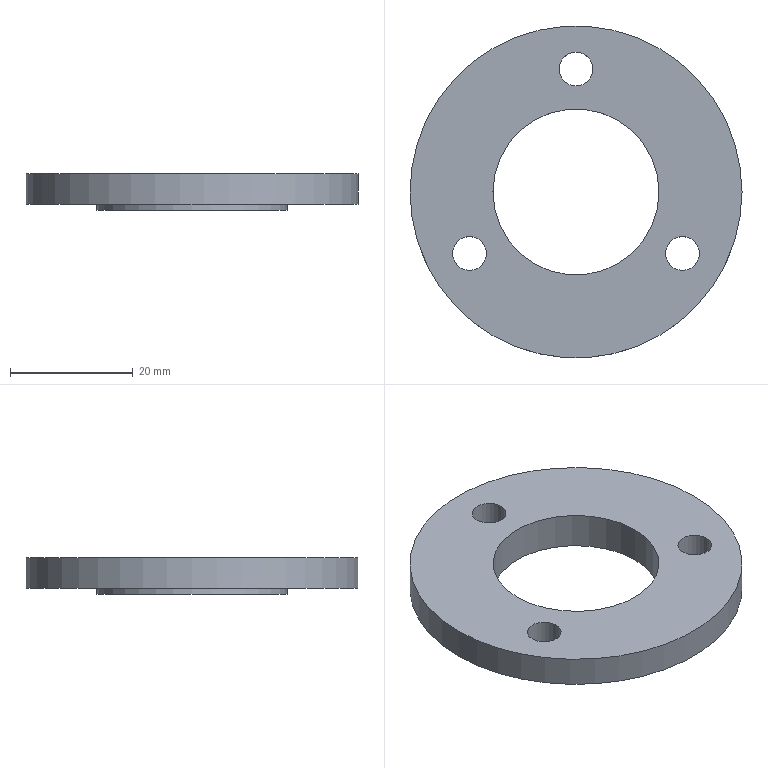Part | STEP file | YBQDJ-YL-15 | 1 solid | 9 faces | box 54 x 54 x 6 mm | volume 8414 mm3 | cylinder 6 | plane 3 | commonest cylinder face diameters 5.5 x3 27 x1 31 x1 54 x1
STEP:
#1=CARTESIAN_POINT('',(0.,0.,0.));
#2=DIRECTION('',(0.,0.,1.));
#3=DIRECTION('',(1.,0.,0.));
#4=AXIS2_PLACEMENT_3D('',#1,#2,#3);
#5=CARTESIAN_POINT('',(291.,-195.,214.));
#6=VERTEX_POINT('',#5);
#7=CARTESIAN_POINT('',(306.5,-195.,214.));
#8=DIRECTION('',(0.,0.,1.));
#9=DIRECTION('',(-1.,0.,0.));
#10=AXIS2_PLACEMENT_3D('',#7,#8,#9);
#11=CIRCLE('',#10,15.5);
#12=CARTESIAN_POINT('',(306.5,-195.,214.));
#13=DIRECTION('',(0.,0.,1.));
#14=DIRECTION('',(-1.,0.,0.));
#15=AXIS2_PLACEMENT_3D('',#12,#13,#14);
#16=PLANE('',#15);
#17=CARTESIAN_POINT('',(0.,0.));
#18=DIRECTION('',(1.,0.));
#19=AXIS2_PLACEMENT_2D('',#17,#18);
#20=CIRCLE('',#19,15.5);
#21=(GEOMETRIC_REPRESENTATION_CONTEXT(2)PARAMETRIC_REPRESENTATION_CONTEXT()REPRESENTATION_CONTEXT('',''));
#22=DEFINITIONAL_REPRESENTATION('',(#20),#21);
#23=PCURVE('',#16,#22);
#24=CARTESIAN_POINT('',(306.5,-195.,214.));
#25=DIRECTION('',(0.,0.,-1.));
#26=DIRECTION('',(-1.,0.,0.));
#27=AXIS2_PLACEMENT_3D('',#24,#25,#26);
#28=CYLINDRICAL_SURFACE('',#27,15.5);
#29=CARTESIAN_POINT('',(6.283,0.));
#30=DIRECTION('',(-1.,0.));
#31=VECTOR('',#30,1.);
#32=LINE('',#29,#31);
#33=(GEOMETRIC_REPRESENTATION_CONTEXT(2)PARAMETRIC_REPRESENTATION_CONTEXT()REPRESENTATION_CONTEXT('',''));
#34=DEFINITIONAL_REPRESENTATION('',(#32),#33);
#35=PCURVE('',#28,#34);
#36=SURFACE_CURVE('',#11,(#23,#35),.PCURVE_S1.);
#37=EDGE_CURVE('',#6,#6,#36,.T.);
#38=ORIENTED_EDGE('',*,*,#37,.T.);
#39=EDGE_LOOP('',(#38));
#40=FACE_BOUND('',#39,.T.);
#41=CARTESIAN_POINT('',(303.75,-175.,214.));
#42=VERTEX_POINT('',#41);
#43=CARTESIAN_POINT('',(306.5,-175.,214.));
#44=DIRECTION('',(0.,0.,1.));
#45=DIRECTION('',(-1.,0.,0.));
#46=AXIS2_PLACEMENT_3D('',#43,#44,#45);
#47=CIRCLE('',#46,2.75);
#48=CARTESIAN_POINT('',(0.,-20.));
#49=DIRECTION('',(1.,0.));
#50=AXIS2_PLACEMENT_2D('',#48,#49);
#51=CIRCLE('',#50,2.75);
#52=(GEOMETRIC_REPRESENTATION_CONTEXT(2)PARAMETRIC_REPRESENTATION_CONTEXT()REPRESENTATION_CONTEXT('',''));
#53=DEFINITIONAL_REPRESENTATION('',(#51),#52);
#54=PCURVE('',#16,#53);
#55=CARTESIAN_POINT('',(306.5,-175.,224.));
#56=DIRECTION('',(0.,0.,-1.));
#57=DIRECTION('',(1.,0.,0.));
#58=AXIS2_PLACEMENT_3D('',#55,#56,#57);
#59=CYLINDRICAL_SURFACE('',#58,2.75);
#60=CARTESIAN_POINT('',(9.425,10.));
#61=DIRECTION('',(-1.,0.));
#62=VECTOR('',#61,1.);
#63=LINE('',#60,#62);
#64=(GEOMETRIC_REPRESENTATION_CONTEXT(2)PARAMETRIC_REPRESENTATION_CONTEXT()REPRESENTATION_CONTEXT('',''));
#65=DEFINITIONAL_REPRESENTATION('',(#63),#64);
#66=PCURVE('',#59,#65);
#67=SURFACE_CURVE('',#47,(#54,#66),.PCURVE_S1.);
#68=EDGE_CURVE('',#42,#42,#67,.T.);
#69=ORIENTED_EDGE('',*,*,#68,.T.);
#70=EDGE_LOOP('',(#69));
#71=FACE_BOUND('',#70,.T.);
#72=CARTESIAN_POINT('',(286.429,-205.,214.));
#73=VERTEX_POINT('',#72);
#74=CARTESIAN_POINT('',(289.179,-205.,214.));
#75=DIRECTION('',(0.,0.,1.));
#76=DIRECTION('',(-1.,0.,0.));
#77=AXIS2_PLACEMENT_3D('',#74,#75,#76);
#78=CIRCLE('',#77,2.75);
#79=CARTESIAN_POINT('',(17.321,10.));
#80=DIRECTION('',(1.,0.));
#81=AXIS2_PLACEMENT_2D('',#79,#80);
#82=CIRCLE('',#81,2.75);
#83=(GEOMETRIC_REPRESENTATION_CONTEXT(2)PARAMETRIC_REPRESENTATION_CONTEXT()REPRESENTATION_CONTEXT('',''));
#84=DEFINITIONAL_REPRESENTATION('',(#82),#83);
#85=PCURVE('',#16,#84);
#86=CARTESIAN_POINT('',(289.179,-205.,224.));
#87=DIRECTION('',(0.,0.,-1.));
#88=DIRECTION('',(1.,0.,0.));
#89=AXIS2_PLACEMENT_3D('',#86,#87,#88);
#90=CYLINDRICAL_SURFACE('',#89,2.75);
#91=CARTESIAN_POINT('',(9.425,10.));
#92=DIRECTION('',(-1.,0.));
#93=VECTOR('',#92,1.);
#94=LINE('',#91,#93);
#95=(GEOMETRIC_REPRESENTATION_CONTEXT(2)PARAMETRIC_REPRESENTATION_CONTEXT()REPRESENTATION_CONTEXT('',''));
#96=DEFINITIONAL_REPRESENTATION('',(#94),#95);
#97=PCURVE('',#90,#96);
#98=SURFACE_CURVE('',#78,(#85,#97),.PCURVE_S1.);
#99=EDGE_CURVE('',#73,#73,#98,.T.);
#100=ORIENTED_EDGE('',*,*,#99,.T.);
#101=EDGE_LOOP('',(#100));
#102=FACE_BOUND('',#101,.T.);
#103=CARTESIAN_POINT('',(321.071,-205.,214.));
#104=VERTEX_POINT('',#103);
#105=CARTESIAN_POINT('',(323.821,-205.,214.));
#106=DIRECTION('',(0.,0.,1.));
#107=DIRECTION('',(-1.,0.,0.));
#108=AXIS2_PLACEMENT_3D('',#105,#106,#107);
#109=CIRCLE('',#108,2.75);
#110=CARTESIAN_POINT('',(-17.321,10.));
#111=DIRECTION('',(1.,0.));
#112=AXIS2_PLACEMENT_2D('',#110,#111);
#113=CIRCLE('',#112,2.75);
#114=(GEOMETRIC_REPRESENTATION_CONTEXT(2)PARAMETRIC_REPRESENTATION_CONTEXT()REPRESENTATION_CONTEXT('',''));
#115=DEFINITIONAL_REPRESENTATION('',(#113),#114);
#116=PCURVE('',#16,#115);
#117=CARTESIAN_POINT('',(323.821,-205.,224.));
#118=DIRECTION('',(0.,0.,-1.));
#119=DIRECTION('',(1.,0.,0.));
#120=AXIS2_PLACEMENT_3D('',#117,#118,#119);
#121=CYLINDRICAL_SURFACE('',#120,2.75);
#122=CARTESIAN_POINT('',(9.425,10.));
#123=DIRECTION('',(-1.,0.));
#124=VECTOR('',#123,1.);
#125=LINE('',#122,#124);
#126=(GEOMETRIC_REPRESENTATION_CONTEXT(2)PARAMETRIC_REPRESENTATION_CONTEXT()REPRESENTATION_CONTEXT('',''));
#127=DEFINITIONAL_REPRESENTATION('',(#125),#126);
#128=PCURVE('',#121,#127);
#129=SURFACE_CURVE('',#109,(#116,#128),.PCURVE_S1.);
#130=EDGE_CURVE('',#104,#104,#129,.T.);
#131=ORIENTED_EDGE('',*,*,#130,.T.);
#132=EDGE_LOOP('',(#131));
#133=FACE_BOUND('',#132,.T.);
#134=CARTESIAN_POINT('',(333.5,-195.,214.));
#135=VERTEX_POINT('',#134);
#136=CARTESIAN_POINT('',(306.5,-195.,214.));
#137=DIRECTION('',(0.,0.,-1.));
#138=DIRECTION('',(1.,0.,0.));
#139=AXIS2_PLACEMENT_3D('',#136,#137,#138);
#140=CIRCLE('',#139,27.);
#141=CARTESIAN_POINT('',(-27.,0.));
#142=CARTESIAN_POINT('',(-27.,46.765));
#143=CARTESIAN_POINT('',(13.5,23.383));
#144=CARTESIAN_POINT('',(54.,0.));
#145=CARTESIAN_POINT('',(13.5,-23.383));
#146=CARTESIAN_POINT('',(-27.,-46.765));
#147=CARTESIAN_POINT('',(-27.,0.));
#148=(BOUNDED_CURVE()B_SPLINE_CURVE(2,(#141,#142,#143,#144,#145,#146,#147),.UNSPECIFIED.,.T.,.F.)B_SPLINE_CURVE_WITH_KNOTS((1,2,2,2,2,1),(-2.094,0.,2.094,4.189,6.283,8.378),.UNSPECIFIED.)CURVE()GEOMETRIC_REPRESENTATION_ITEM()RATIONAL_B_SPLINE_CURVE((1.,0.5,1.,0.5,1.,0.5,1.))REPRESENTATION_ITEM(''));
#149=(GEOMETRIC_REPRESENTATION_CONTEXT(2)PARAMETRIC_REPRESENTATION_CONTEXT()REPRESENTATION_CONTEXT('',''));
#150=DEFINITIONAL_REPRESENTATION('',(#148),#149);
#151=PCURVE('',#16,#150);
#152=CARTESIAN_POINT('',(306.5,-195.,214.));
#153=DIRECTION('',(0.,0.,1.));
#154=DIRECTION('',(-1.,0.,0.));
#155=AXIS2_PLACEMENT_3D('',#152,#153,#154);
#156=CYLINDRICAL_SURFACE('',#155,27.);
#157=CARTESIAN_POINT('',(9.425,0.));
#158=DIRECTION('',(-1.,0.));
#159=VECTOR('',#158,1.);
#160=LINE('',#157,#159);
#161=(GEOMETRIC_REPRESENTATION_CONTEXT(2)PARAMETRIC_REPRESENTATION_CONTEXT()REPRESENTATION_CONTEXT('',''));
#162=DEFINITIONAL_REPRESENTATION('',(#160),#161);
#163=PCURVE('',#156,#162);
#164=SURFACE_CURVE('',#140,(#151,#163),.PCURVE_S1.);
#165=EDGE_CURVE('',#135,#135,#164,.T.);
#166=ORIENTED_EDGE('',*,*,#165,.T.);
#167=EDGE_LOOP('',(#166));
#168=FACE_BOUND('',#167,.T.);
#169=ADVANCED_FACE('',(#40,#71,#102,#133,#168),#16,.F.);
#170=CARTESIAN_POINT('',(303.75,-175.,219.));
#171=VERTEX_POINT('',#170);
#172=CARTESIAN_POINT('',(306.5,-175.,219.));
#173=DIRECTION('',(0.,0.,-1.));
#174=DIRECTION('',(-1.,0.,0.));
#175=AXIS2_PLACEMENT_3D('',#172,#173,#174);
#176=CIRCLE('',#175,2.75);
#177=CARTESIAN_POINT('',(306.5,-195.,219.));
#178=DIRECTION('',(0.,0.,1.));
#179=DIRECTION('',(-1.,0.,0.));
#180=AXIS2_PLACEMENT_3D('',#177,#178,#179);
#181=PLANE('',#180);
#182=CARTESIAN_POINT('',(2.75,-20.));
#183=CARTESIAN_POINT('',(2.75,-24.763));
#184=CARTESIAN_POINT('',(-1.375,-22.382));
#185=CARTESIAN_POINT('',(-5.5,-20.));
#186=CARTESIAN_POINT('',(-1.375,-17.618));
#187=CARTESIAN_POINT('',(2.75,-15.237));
#188=CARTESIAN_POINT('',(2.75,-20.));
#189=(BOUNDED_CURVE()B_SPLINE_CURVE(2,(#182,#183,#184,#185,#186,#187,#188),.UNSPECIFIED.,.T.,.F.)B_SPLINE_CURVE_WITH_KNOTS((1,2,2,2,2,1),(-2.094,0.,2.094,4.189,6.283,8.378),.UNSPECIFIED.)CURVE()GEOMETRIC_REPRESENTATION_ITEM()RATIONAL_B_SPLINE_CURVE((1.,0.5,1.,0.5,1.,0.5,1.))REPRESENTATION_ITEM(''));
#190=(GEOMETRIC_REPRESENTATION_CONTEXT(2)PARAMETRIC_REPRESENTATION_CONTEXT()REPRESENTATION_CONTEXT('',''));
#191=DEFINITIONAL_REPRESENTATION('',(#189),#190);
#192=PCURVE('',#181,#191);
#193=CARTESIAN_POINT('',(3.142,5.));
#194=DIRECTION('',(1.,0.));
#195=VECTOR('',#194,1.);
#196=LINE('',#193,#195);
#197=(GEOMETRIC_REPRESENTATION_CONTEXT(2)PARAMETRIC_REPRESENTATION_CONTEXT()REPRESENTATION_CONTEXT('',''));
#198=DEFINITIONAL_REPRESENTATION('',(#196),#197);
#199=PCURVE('',#59,#198);
#200=SURFACE_CURVE('',#176,(#192,#199),.PCURVE_S1.);
#201=EDGE_CURVE('',#171,#171,#200,.T.);
#202=ORIENTED_EDGE('',*,*,#201,.T.);
#203=EDGE_LOOP('',(#202));
#204=FACE_BOUND('',#203,.T.);
#205=CARTESIAN_POINT('',(286.429,-205.,219.));
#206=VERTEX_POINT('',#205);
#207=CARTESIAN_POINT('',(289.179,-205.,219.));
#208=DIRECTION('',(0.,0.,-1.));
#209=DIRECTION('',(-1.,0.,0.));
#210=AXIS2_PLACEMENT_3D('',#207,#208,#209);
#211=CIRCLE('',#210,2.75);
#212=CARTESIAN_POINT('',(20.071,10.));
#213=CARTESIAN_POINT('',(20.071,5.237));
#214=CARTESIAN_POINT('',(15.946,7.618));
#215=CARTESIAN_POINT('',(11.821,10.));
#216=CARTESIAN_POINT('',(15.946,12.382));
#217=CARTESIAN_POINT('',(20.071,14.763));
#218=CARTESIAN_POINT('',(20.071,10.));
#219=(BOUNDED_CURVE()B_SPLINE_CURVE(2,(#212,#213,#214,#215,#216,#217,#218),.UNSPECIFIED.,.T.,.F.)B_SPLINE_CURVE_WITH_KNOTS((1,2,2,2,2,1),(-2.094,0.,2.094,4.189,6.283,8.378),.UNSPECIFIED.)CURVE()GEOMETRIC_REPRESENTATION_ITEM()RATIONAL_B_SPLINE_CURVE((1.,0.5,1.,0.5,1.,0.5,1.))REPRESENTATION_ITEM(''));
#220=(GEOMETRIC_REPRESENTATION_CONTEXT(2)PARAMETRIC_REPRESENTATION_CONTEXT()REPRESENTATION_CONTEXT('',''));
#221=DEFINITIONAL_REPRESENTATION('',(#219),#220);
#222=PCURVE('',#181,#221);
#223=CARTESIAN_POINT('',(3.142,5.));
#224=DIRECTION('',(1.,0.));
#225=VECTOR('',#224,1.);
#226=LINE('',#223,#225);
#227=(GEOMETRIC_REPRESENTATION_CONTEXT(2)PARAMETRIC_REPRESENTATION_CONTEXT()REPRESENTATION_CONTEXT('',''));
#228=DEFINITIONAL_REPRESENTATION('',(#226),#227);
#229=PCURVE('',#90,#228);
#230=SURFACE_CURVE('',#211,(#222,#229),.PCURVE_S1.);
#231=EDGE_CURVE('',#206,#206,#230,.T.);
#232=ORIENTED_EDGE('',*,*,#231,.T.);
#233=EDGE_LOOP('',(#232));
#234=FACE_BOUND('',#233,.T.);
#235=CARTESIAN_POINT('',(321.071,-205.,219.));
#236=VERTEX_POINT('',#235);
#237=CARTESIAN_POINT('',(323.821,-205.,219.));
#238=DIRECTION('',(0.,0.,-1.));
#239=DIRECTION('',(-1.,0.,0.));
#240=AXIS2_PLACEMENT_3D('',#237,#238,#239);
#241=CIRCLE('',#240,2.75);
#242=CARTESIAN_POINT('',(-14.571,10.));
#243=CARTESIAN_POINT('',(-14.571,5.237));
#244=CARTESIAN_POINT('',(-18.696,7.618));
#245=CARTESIAN_POINT('',(-22.821,10.));
#246=CARTESIAN_POINT('',(-18.696,12.382));
#247=CARTESIAN_POINT('',(-14.571,14.763));
#248=CARTESIAN_POINT('',(-14.571,10.));
#249=(BOUNDED_CURVE()B_SPLINE_CURVE(2,(#242,#243,#244,#245,#246,#247,#248),.UNSPECIFIED.,.T.,.F.)B_SPLINE_CURVE_WITH_KNOTS((1,2,2,2,2,1),(-2.094,0.,2.094,4.189,6.283,8.378),.UNSPECIFIED.)CURVE()GEOMETRIC_REPRESENTATION_ITEM()RATIONAL_B_SPLINE_CURVE((1.,0.5,1.,0.5,1.,0.5,1.))REPRESENTATION_ITEM(''));
#250=(GEOMETRIC_REPRESENTATION_CONTEXT(2)PARAMETRIC_REPRESENTATION_CONTEXT()REPRESENTATION_CONTEXT('',''));
#251=DEFINITIONAL_REPRESENTATION('',(#249),#250);
#252=PCURVE('',#181,#251);
#253=CARTESIAN_POINT('',(3.142,5.));
#254=DIRECTION('',(1.,0.));
#255=VECTOR('',#254,1.);
#256=LINE('',#253,#255);
#257=(GEOMETRIC_REPRESENTATION_CONTEXT(2)PARAMETRIC_REPRESENTATION_CONTEXT()REPRESENTATION_CONTEXT('',''));
#258=DEFINITIONAL_REPRESENTATION('',(#256),#257);
#259=PCURVE('',#121,#258);
#260=SURFACE_CURVE('',#241,(#252,#259),.PCURVE_S1.);
#261=EDGE_CURVE('',#236,#236,#260,.T.);
#262=ORIENTED_EDGE('',*,*,#261,.T.);
#263=EDGE_LOOP('',(#262));
#264=FACE_BOUND('',#263,.T.);
#265=CARTESIAN_POINT('',(333.5,-195.,219.));
#266=VERTEX_POINT('',#265);
#267=CARTESIAN_POINT('',(306.5,-195.,219.));
#268=DIRECTION('',(0.,0.,-1.));
#269=DIRECTION('',(1.,0.,0.));
#270=AXIS2_PLACEMENT_3D('',#267,#268,#269);
#271=CIRCLE('',#270,27.);
#272=CARTESIAN_POINT('',(-27.,0.));
#273=CARTESIAN_POINT('',(-27.,46.765));
#274=CARTESIAN_POINT('',(13.5,23.383));
#275=CARTESIAN_POINT('',(54.,0.));
#276=CARTESIAN_POINT('',(13.5,-23.383));
#277=CARTESIAN_POINT('',(-27.,-46.765));
#278=CARTESIAN_POINT('',(-27.,0.));
#279=(BOUNDED_CURVE()B_SPLINE_CURVE(2,(#272,#273,#274,#275,#276,#277,#278),.UNSPECIFIED.,.T.,.F.)B_SPLINE_CURVE_WITH_KNOTS((1,2,2,2,2,1),(-2.094,0.,2.094,4.189,6.283,8.378),.UNSPECIFIED.)CURVE()GEOMETRIC_REPRESENTATION_ITEM()RATIONAL_B_SPLINE_CURVE((1.,0.5,1.,0.5,1.,0.5,1.))REPRESENTATION_ITEM(''));
#280=(GEOMETRIC_REPRESENTATION_CONTEXT(2)PARAMETRIC_REPRESENTATION_CONTEXT()REPRESENTATION_CONTEXT('',''));
#281=DEFINITIONAL_REPRESENTATION('',(#279),#280);
#282=PCURVE('',#181,#281);
#283=CARTESIAN_POINT('',(9.425,5.));
#284=DIRECTION('',(-1.,0.));
#285=VECTOR('',#284,1.);
#286=LINE('',#283,#285);
#287=(GEOMETRIC_REPRESENTATION_CONTEXT(2)PARAMETRIC_REPRESENTATION_CONTEXT()REPRESENTATION_CONTEXT('',''));
#288=DEFINITIONAL_REPRESENTATION('',(#286),#287);
#289=PCURVE('',#156,#288);
#290=SURFACE_CURVE('',#271,(#282,#289),.PCURVE_S1.);
#291=EDGE_CURVE('',#266,#266,#290,.T.);
#292=ORIENTED_EDGE('',*,*,#291,.F.);
#293=EDGE_LOOP('',(#292));
#294=FACE_BOUND('',#293,.T.);
#295=CARTESIAN_POINT('',(320.,-195.,219.));
#296=VERTEX_POINT('',#295);
#297=CARTESIAN_POINT('',(293.,-195.,219.));
#298=VERTEX_POINT('',#297);
#299=CARTESIAN_POINT('',(306.5,-195.,219.));
#300=DIRECTION('',(0.,0.,-1.));
#301=DIRECTION('',(1.,0.,0.));
#302=AXIS2_PLACEMENT_3D('',#299,#300,#301);
#303=CIRCLE('',#302,13.5);
#304=CARTESIAN_POINT('',(-13.5,0.));
#305=CARTESIAN_POINT('',(-13.5,23.383));
#306=CARTESIAN_POINT('',(6.75,11.691));
#307=CARTESIAN_POINT('',(27.,0.));
#308=CARTESIAN_POINT('',(6.75,-11.691));
#309=CARTESIAN_POINT('',(-13.5,-23.383));
#310=CARTESIAN_POINT('',(-13.5,0.));
#311=(BOUNDED_CURVE()B_SPLINE_CURVE(2,(#304,#305,#306,#307,#308,#309,#310),.UNSPECIFIED.,.T.,.F.)B_SPLINE_CURVE_WITH_KNOTS((1,2,2,2,2,1),(-2.094,0.,2.094,4.189,6.283,8.378),.UNSPECIFIED.)CURVE()GEOMETRIC_REPRESENTATION_ITEM()RATIONAL_B_SPLINE_CURVE((1.,0.5,1.,0.5,1.,0.5,1.))REPRESENTATION_ITEM(''));
#312=(GEOMETRIC_REPRESENTATION_CONTEXT(2)PARAMETRIC_REPRESENTATION_CONTEXT()REPRESENTATION_CONTEXT('',''));
#313=DEFINITIONAL_REPRESENTATION('',(#311),#312);
#314=PCURVE('',#181,#313);
#315=CARTESIAN_POINT('',(306.5,-195.,214.));
#316=DIRECTION('',(0.,0.,1.));
#317=DIRECTION('',(-1.,0.,0.));
#318=AXIS2_PLACEMENT_3D('',#315,#316,#317);
#319=CYLINDRICAL_SURFACE('',#318,13.5);
#320=CARTESIAN_POINT('',(3.142,5.));
#321=DIRECTION('',(-1.,0.));
#322=VECTOR('',#321,1.);
#323=LINE('',#320,#322);
#324=(GEOMETRIC_REPRESENTATION_CONTEXT(2)PARAMETRIC_REPRESENTATION_CONTEXT()REPRESENTATION_CONTEXT('',''));
#325=DEFINITIONAL_REPRESENTATION('',(#323),#324);
#326=PCURVE('',#319,#325);
#327=SURFACE_CURVE('',#303,(#314,#326),.PCURVE_S1.);
#328=EDGE_CURVE('',#296,#298,#327,.T.);
#329=ORIENTED_EDGE('',*,*,#328,.T.);
#330=CARTESIAN_POINT('',(306.5,-195.,219.));
#331=DIRECTION('',(0.,0.,-1.));
#332=DIRECTION('',(1.,0.,0.));
#333=AXIS2_PLACEMENT_3D('',#330,#331,#332);
#334=CIRCLE('',#333,13.5);
#335=CARTESIAN_POINT('',(-13.5,0.));
#336=CARTESIAN_POINT('',(-13.5,23.383));
#337=CARTESIAN_POINT('',(6.75,11.691));
#338=CARTESIAN_POINT('',(27.,0.));
#339=CARTESIAN_POINT('',(6.75,-11.691));
#340=CARTESIAN_POINT('',(-13.5,-23.383));
#341=CARTESIAN_POINT('',(-13.5,0.));
#342=(BOUNDED_CURVE()B_SPLINE_CURVE(2,(#335,#336,#337,#338,#339,#340,#341),.UNSPECIFIED.,.T.,.F.)B_SPLINE_CURVE_WITH_KNOTS((1,2,2,2,2,1),(-2.094,0.,2.094,4.189,6.283,8.378),.UNSPECIFIED.)CURVE()GEOMETRIC_REPRESENTATION_ITEM()RATIONAL_B_SPLINE_CURVE((1.,0.5,1.,0.5,1.,0.5,1.))REPRESENTATION_ITEM(''));
#343=(GEOMETRIC_REPRESENTATION_CONTEXT(2)PARAMETRIC_REPRESENTATION_CONTEXT()REPRESENTATION_CONTEXT('',''));
#344=DEFINITIONAL_REPRESENTATION('',(#342),#343);
#345=PCURVE('',#181,#344);
#346=CARTESIAN_POINT('',(9.425,5.));
#347=DIRECTION('',(-1.,0.));
#348=VECTOR('',#347,1.);
#349=LINE('',#346,#348);
#350=(GEOMETRIC_REPRESENTATION_CONTEXT(2)PARAMETRIC_REPRESENTATION_CONTEXT()REPRESENTATION_CONTEXT('',''));
#351=DEFINITIONAL_REPRESENTATION('',(#349),#350);
#352=PCURVE('',#319,#351);
#353=SURFACE_CURVE('',#334,(#345,#352),.PCURVE_S1.);
#354=EDGE_CURVE('',#298,#296,#353,.T.);
#355=ORIENTED_EDGE('',*,*,#354,.T.);
#356=EDGE_LOOP('',(#329,#355));
#357=FACE_BOUND('',#356,.T.);
#358=ADVANCED_FACE('',(#204,#234,#264,#294,#357),#181,.T.);
#359=ORIENTED_EDGE('',*,*,#165,.F.);
#360=CARTESIAN_POINT('',(333.5,-195.,214.));
#361=CARTESIAN_POINT('',(333.5,-195.,219.));
#362=B_SPLINE_CURVE_WITH_KNOTS('',1,(#360,#361),.UNSPECIFIED.,.F.,.F.,(2,2),(0.,5.),.PIECEWISE_BEZIER_KNOTS.);
#363=CARTESIAN_POINT('',(9.425,0.));
#364=DIRECTION('',(0.,1.));
#365=VECTOR('',#364,1.);
#366=LINE('',#363,#365);
#367=(GEOMETRIC_REPRESENTATION_CONTEXT(2)PARAMETRIC_REPRESENTATION_CONTEXT()REPRESENTATION_CONTEXT('',''));
#368=DEFINITIONAL_REPRESENTATION('',(#366),#367);
#369=PCURVE('',#156,#368);
#370=CARTESIAN_POINT('',(3.142,0.));
#371=DIRECTION('',(0.,1.));
#372=VECTOR('',#371,1.);
#373=LINE('',#370,#372);
#374=(GEOMETRIC_REPRESENTATION_CONTEXT(2)PARAMETRIC_REPRESENTATION_CONTEXT()REPRESENTATION_CONTEXT('',''));
#375=DEFINITIONAL_REPRESENTATION('',(#373),#374);
#376=PCURVE('',#156,#375);
#377=SEAM_CURVE('',#362,(#369,#376),.PCURVE_S1.);
#378=EDGE_CURVE('',#135,#266,#377,.T.);
#379=ORIENTED_EDGE('',*,*,#378,.T.);
#380=ORIENTED_EDGE('',*,*,#291,.T.);
#381=ORIENTED_EDGE('',*,*,#378,.F.);
#382=EDGE_LOOP('',(#359,#379,#380,#381));
#383=FACE_BOUND('',#382,.T.);
#384=ADVANCED_FACE('',(#383),#156,.T.);
#385=ORIENTED_EDGE('',*,*,#328,.T.);
#386=CARTESIAN_POINT('',(293.,-195.,213.));
#387=VERTEX_POINT('',#386);
#388=CARTESIAN_POINT('',(293.,-195.,213.));
#389=CARTESIAN_POINT('',(293.,-195.,219.));
#390=B_SPLINE_CURVE_WITH_KNOTS('',1,(#388,#389),.UNSPECIFIED.,.F.,.F.,(2,2),(-1.,5.),.PIECEWISE_BEZIER_KNOTS.);
#391=CARTESIAN_POINT('',(0.,0.));
#392=DIRECTION('',(0.,1.));
#393=VECTOR('',#392,1.);
#394=LINE('',#391,#393);
#395=(GEOMETRIC_REPRESENTATION_CONTEXT(2)PARAMETRIC_REPRESENTATION_CONTEXT()REPRESENTATION_CONTEXT('',''));
#396=DEFINITIONAL_REPRESENTATION('',(#394),#395);
#397=PCURVE('',#319,#396);
#398=CARTESIAN_POINT('',(6.283,0.));
#399=DIRECTION('',(0.,1.));
#400=VECTOR('',#399,1.);
#401=LINE('',#398,#400);
#402=(GEOMETRIC_REPRESENTATION_CONTEXT(2)PARAMETRIC_REPRESENTATION_CONTEXT()REPRESENTATION_CONTEXT('',''));
#403=DEFINITIONAL_REPRESENTATION('',(#401),#402);
#404=PCURVE('',#319,#403);
#405=SEAM_CURVE('',#390,(#397,#404),.PCURVE_S1.);
#406=EDGE_CURVE('',#387,#298,#405,.T.);
#407=ORIENTED_EDGE('',*,*,#406,.F.);
#408=CARTESIAN_POINT('',(306.5,-195.,213.));
#409=DIRECTION('',(0.,0.,1.));
#410=DIRECTION('',(-1.,0.,0.));
#411=AXIS2_PLACEMENT_3D('',#408,#409,#410);
#412=CIRCLE('',#411,13.5);
#413=CARTESIAN_POINT('',(0.,-1.));
#414=DIRECTION('',(1.,0.));
#415=VECTOR('',#414,1.);
#416=LINE('',#413,#415);
#417=(GEOMETRIC_REPRESENTATION_CONTEXT(2)PARAMETRIC_REPRESENTATION_CONTEXT()REPRESENTATION_CONTEXT('',''));
#418=DEFINITIONAL_REPRESENTATION('',(#416),#417);
#419=PCURVE('',#319,#418);
#420=CARTESIAN_POINT('',(306.5,-195.,213.));
#421=DIRECTION('',(0.,0.,-1.));
#422=DIRECTION('',(-1.,0.,0.));
#423=AXIS2_PLACEMENT_3D('',#420,#421,#422);
#424=PLANE('',#423);
#425=CARTESIAN_POINT('',(13.5,0.));
#426=CARTESIAN_POINT('',(13.5,-23.383));
#427=CARTESIAN_POINT('',(-6.75,-11.691));
#428=CARTESIAN_POINT('',(-27.,0.));
#429=CARTESIAN_POINT('',(-6.75,11.691));
#430=CARTESIAN_POINT('',(13.5,23.383));
#431=CARTESIAN_POINT('',(13.5,0.));
#432=(BOUNDED_CURVE()B_SPLINE_CURVE(2,(#425,#426,#427,#428,#429,#430,#431),.UNSPECIFIED.,.T.,.F.)B_SPLINE_CURVE_WITH_KNOTS((1,2,2,2,2,1),(-2.094,0.,2.094,4.189,6.283,8.378),.UNSPECIFIED.)CURVE()GEOMETRIC_REPRESENTATION_ITEM()RATIONAL_B_SPLINE_CURVE((1.,0.5,1.,0.5,1.,0.5,1.))REPRESENTATION_ITEM(''));
#433=(GEOMETRIC_REPRESENTATION_CONTEXT(2)PARAMETRIC_REPRESENTATION_CONTEXT()REPRESENTATION_CONTEXT('',''));
#434=DEFINITIONAL_REPRESENTATION('',(#432),#433);
#435=PCURVE('',#424,#434);
#436=SURFACE_CURVE('',#412,(#419,#435),.PCURVE_S1.);
#437=EDGE_CURVE('',#387,#387,#436,.T.);
#438=ORIENTED_EDGE('',*,*,#437,.T.);
#439=ORIENTED_EDGE('',*,*,#406,.T.);
#440=ORIENTED_EDGE('',*,*,#354,.T.);
#441=EDGE_LOOP('',(#385,#407,#438,#439,#440));
#442=FACE_BOUND('',#441,.F.);
#443=ADVANCED_FACE('',(#442),#319,.F.);
#444=ORIENTED_EDGE('',*,*,#130,.T.);
#445=CARTESIAN_POINT('',(321.071,-205.,219.));
#446=CARTESIAN_POINT('',(321.071,-205.,214.));
#447=B_SPLINE_CURVE_WITH_KNOTS('',1,(#445,#446),.UNSPECIFIED.,.F.,.F.,(2,2),(5.,10.),.PIECEWISE_BEZIER_KNOTS.);
#448=CARTESIAN_POINT('',(3.142,0.));
#449=DIRECTION('',(0.,1.));
#450=VECTOR('',#449,1.);
#451=LINE('',#448,#450);
#452=(GEOMETRIC_REPRESENTATION_CONTEXT(2)PARAMETRIC_REPRESENTATION_CONTEXT()REPRESENTATION_CONTEXT('',''));
#453=DEFINITIONAL_REPRESENTATION('',(#451),#452);
#454=PCURVE('',#121,#453);
#455=CARTESIAN_POINT('',(9.425,0.));
#456=DIRECTION('',(0.,1.));
#457=VECTOR('',#456,1.);
#458=LINE('',#455,#457);
#459=(GEOMETRIC_REPRESENTATION_CONTEXT(2)PARAMETRIC_REPRESENTATION_CONTEXT()REPRESENTATION_CONTEXT('',''));
#460=DEFINITIONAL_REPRESENTATION('',(#458),#459);
#461=PCURVE('',#121,#460);
#462=SEAM_CURVE('',#447,(#454,#461),.PCURVE_S1.);
#463=EDGE_CURVE('',#236,#104,#462,.T.);
#464=ORIENTED_EDGE('',*,*,#463,.F.);
#465=ORIENTED_EDGE('',*,*,#261,.T.);
#466=ORIENTED_EDGE('',*,*,#463,.T.);
#467=EDGE_LOOP('',(#444,#464,#465,#466));
#468=FACE_BOUND('',#467,.F.);
#469=ADVANCED_FACE('',(#468),#121,.F.);
#470=ORIENTED_EDGE('',*,*,#99,.T.);
#471=CARTESIAN_POINT('',(286.429,-205.,219.));
#472=CARTESIAN_POINT('',(286.429,-205.,214.));
#473=B_SPLINE_CURVE_WITH_KNOTS('',1,(#471,#472),.UNSPECIFIED.,.F.,.F.,(2,2),(5.,10.),.PIECEWISE_BEZIER_KNOTS.);
#474=CARTESIAN_POINT('',(3.142,0.));
#475=DIRECTION('',(0.,1.));
#476=VECTOR('',#475,1.);
#477=LINE('',#474,#476);
#478=(GEOMETRIC_REPRESENTATION_CONTEXT(2)PARAMETRIC_REPRESENTATION_CONTEXT()REPRESENTATION_CONTEXT('',''));
#479=DEFINITIONAL_REPRESENTATION('',(#477),#478);
#480=PCURVE('',#90,#479);
#481=CARTESIAN_POINT('',(9.425,0.));
#482=DIRECTION('',(0.,1.));
#483=VECTOR('',#482,1.);
#484=LINE('',#481,#483);
#485=(GEOMETRIC_REPRESENTATION_CONTEXT(2)PARAMETRIC_REPRESENTATION_CONTEXT()REPRESENTATION_CONTEXT('',''));
#486=DEFINITIONAL_REPRESENTATION('',(#484),#485);
#487=PCURVE('',#90,#486);
#488=SEAM_CURVE('',#473,(#480,#487),.PCURVE_S1.);
#489=EDGE_CURVE('',#206,#73,#488,.T.);
#490=ORIENTED_EDGE('',*,*,#489,.F.);
#491=ORIENTED_EDGE('',*,*,#231,.T.);
#492=ORIENTED_EDGE('',*,*,#489,.T.);
#493=EDGE_LOOP('',(#470,#490,#491,#492));
#494=FACE_BOUND('',#493,.F.);
#495=ADVANCED_FACE('',(#494),#90,.F.);
#496=ORIENTED_EDGE('',*,*,#68,.T.);
#497=CARTESIAN_POINT('',(303.75,-175.,219.));
#498=CARTESIAN_POINT('',(303.75,-175.,214.));
#499=B_SPLINE_CURVE_WITH_KNOTS('',1,(#497,#498),.UNSPECIFIED.,.F.,.F.,(2,2),(5.,10.),.PIECEWISE_BEZIER_KNOTS.);
#500=CARTESIAN_POINT('',(3.142,0.));
#501=DIRECTION('',(0.,1.));
#502=VECTOR('',#501,1.);
#503=LINE('',#500,#502);
#504=(GEOMETRIC_REPRESENTATION_CONTEXT(2)PARAMETRIC_REPRESENTATION_CONTEXT()REPRESENTATION_CONTEXT('',''));
#505=DEFINITIONAL_REPRESENTATION('',(#503),#504);
#506=PCURVE('',#59,#505);
#507=CARTESIAN_POINT('',(9.425,0.));
#508=DIRECTION('',(0.,1.));
#509=VECTOR('',#508,1.);
#510=LINE('',#507,#509);
#511=(GEOMETRIC_REPRESENTATION_CONTEXT(2)PARAMETRIC_REPRESENTATION_CONTEXT()REPRESENTATION_CONTEXT('',''));
#512=DEFINITIONAL_REPRESENTATION('',(#510),#511);
#513=PCURVE('',#59,#512);
#514=SEAM_CURVE('',#499,(#506,#513),.PCURVE_S1.);
#515=EDGE_CURVE('',#171,#42,#514,.T.);
#516=ORIENTED_EDGE('',*,*,#515,.F.);
#517=ORIENTED_EDGE('',*,*,#201,.T.);
#518=ORIENTED_EDGE('',*,*,#515,.T.);
#519=EDGE_LOOP('',(#496,#516,#517,#518));
#520=FACE_BOUND('',#519,.F.);
#521=ADVANCED_FACE('',(#520),#59,.F.);
#522=CARTESIAN_POINT('',(291.,-195.,213.));
#523=VERTEX_POINT('',#522);
#524=CARTESIAN_POINT('',(306.5,-195.,213.));
#525=DIRECTION('',(0.,0.,1.));
#526=DIRECTION('',(-1.,0.,0.));
#527=AXIS2_PLACEMENT_3D('',#524,#525,#526);
#528=CIRCLE('',#527,15.5);
#529=CARTESIAN_POINT('',(15.5,0.));
#530=CARTESIAN_POINT('',(15.5,-26.847));
#531=CARTESIAN_POINT('',(-7.75,-13.423));
#532=CARTESIAN_POINT('',(-31.,0.));
#533=CARTESIAN_POINT('',(-7.75,13.423));
#534=CARTESIAN_POINT('',(15.5,26.847));
#535=CARTESIAN_POINT('',(15.5,0.));
#536=(BOUNDED_CURVE()B_SPLINE_CURVE(2,(#529,#530,#531,#532,#533,#534,#535),.UNSPECIFIED.,.T.,.F.)B_SPLINE_CURVE_WITH_KNOTS((1,2,2,2,2,1),(-2.094,0.,2.094,4.189,6.283,8.378),.UNSPECIFIED.)CURVE()GEOMETRIC_REPRESENTATION_ITEM()RATIONAL_B_SPLINE_CURVE((1.,0.5,1.,0.5,1.,0.5,1.))REPRESENTATION_ITEM(''));
#537=(GEOMETRIC_REPRESENTATION_CONTEXT(2)PARAMETRIC_REPRESENTATION_CONTEXT()REPRESENTATION_CONTEXT('',''));
#538=DEFINITIONAL_REPRESENTATION('',(#536),#537);
#539=PCURVE('',#424,#538);
#540=CARTESIAN_POINT('',(6.283,1.));
#541=DIRECTION('',(-1.,0.));
#542=VECTOR('',#541,1.);
#543=LINE('',#540,#542);
#544=(GEOMETRIC_REPRESENTATION_CONTEXT(2)PARAMETRIC_REPRESENTATION_CONTEXT()REPRESENTATION_CONTEXT('',''));
#545=DEFINITIONAL_REPRESENTATION('',(#543),#544);
#546=PCURVE('',#28,#545);
#547=SURFACE_CURVE('',#528,(#539,#546),.PCURVE_S1.);
#548=EDGE_CURVE('',#523,#523,#547,.T.);
#549=ORIENTED_EDGE('',*,*,#548,.F.);
#550=EDGE_LOOP('',(#549));
#551=FACE_BOUND('',#550,.T.);
#552=ORIENTED_EDGE('',*,*,#437,.T.);
#553=EDGE_LOOP('',(#552));
#554=FACE_BOUND('',#553,.T.);
#555=ADVANCED_FACE('',(#551,#554),#424,.T.);
#556=ORIENTED_EDGE('',*,*,#37,.F.);
#557=CARTESIAN_POINT('',(291.,-195.,214.));
#558=CARTESIAN_POINT('',(291.,-195.,213.));
#559=B_SPLINE_CURVE_WITH_KNOTS('',1,(#557,#558),.UNSPECIFIED.,.F.,.F.,(2,2),(0.,1.),.PIECEWISE_BEZIER_KNOTS.);
#560=CARTESIAN_POINT('',(6.283,0.));
#561=DIRECTION('',(0.,1.));
#562=VECTOR('',#561,1.);
#563=LINE('',#560,#562);
#564=(GEOMETRIC_REPRESENTATION_CONTEXT(2)PARAMETRIC_REPRESENTATION_CONTEXT()REPRESENTATION_CONTEXT('',''));
#565=DEFINITIONAL_REPRESENTATION('',(#563),#564);
#566=PCURVE('',#28,#565);
#567=CARTESIAN_POINT('',(0.,0.));
#568=DIRECTION('',(0.,1.));
#569=VECTOR('',#568,1.);
#570=LINE('',#567,#569);
#571=(GEOMETRIC_REPRESENTATION_CONTEXT(2)PARAMETRIC_REPRESENTATION_CONTEXT()REPRESENTATION_CONTEXT('',''));
#572=DEFINITIONAL_REPRESENTATION('',(#570),#571);
#573=PCURVE('',#28,#572);
#574=SEAM_CURVE('',#559,(#566,#573),.PCURVE_S1.);
#575=EDGE_CURVE('',#6,#523,#574,.T.);
#576=ORIENTED_EDGE('',*,*,#575,.T.);
#577=ORIENTED_EDGE('',*,*,#548,.T.);
#578=ORIENTED_EDGE('',*,*,#575,.F.);
#579=EDGE_LOOP('',(#556,#576,#577,#578));
#580=FACE_BOUND('',#579,.T.);
#581=ADVANCED_FACE('',(#580),#28,.T.);
#582=CLOSED_SHELL('',(#169,#358,#384,#443,#469,#495,#521,#555,#581));
#583=MANIFOLD_SOLID_BREP('',#582);
#584=(LENGTH_UNIT()NAMED_UNIT(*)SI_UNIT(.MILLI.,.METRE.));
#585=UNCERTAINTY_MEASURE_WITH_UNIT(LENGTH_MEASURE(0.00001),#584,'','');
#586=(NAMED_UNIT(*)PLANE_ANGLE_UNIT()SI_UNIT($,.RADIAN.));
#587=(NAMED_UNIT(*)SI_UNIT($,.STERADIAN.)SOLID_ANGLE_UNIT());
#588=(GEOMETRIC_REPRESENTATION_CONTEXT(3)GLOBAL_UNCERTAINTY_ASSIGNED_CONTEXT((#585))GLOBAL_UNIT_ASSIGNED_CONTEXT((#584,#586,#587))REPRESENTATION_CONTEXT('',''));
#589=ADVANCED_BREP_SHAPE_REPRESENTATION('',(#4,#583),#588);